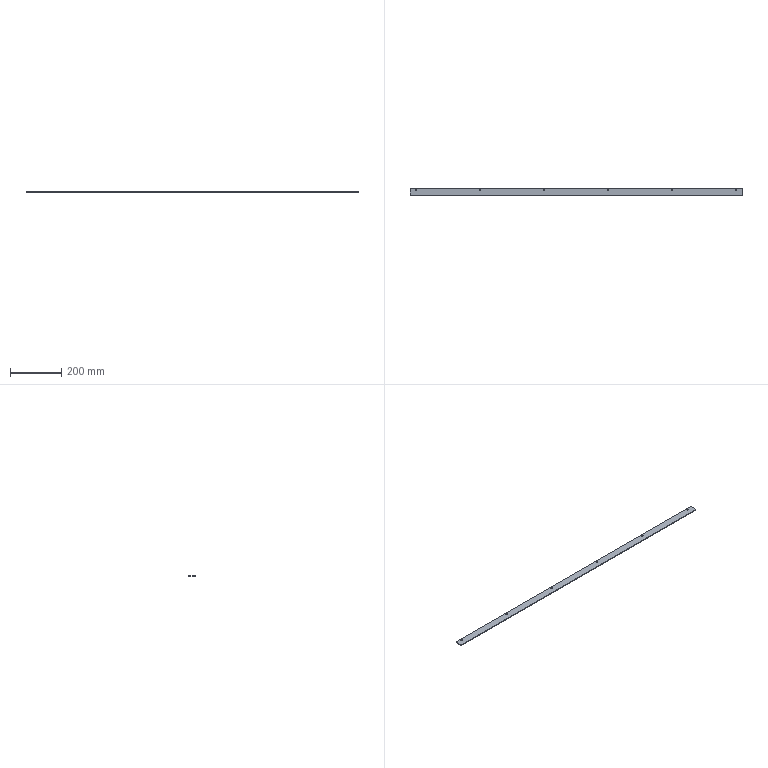Part | NX | features BREP 1 | 1 solid | 34 faces | box 1300 x 30 x 3 mm | volume 116367 mm3 | cone 12 | cylinder 12 | plane 10 | commonest cylinder face diameters 4.8 x12
STEP:
#1=CARTESIAN_POINT('',(648.,-15.,3.));
#2=VERTEX_POINT('',#1);
#3=CARTESIAN_POINT('',(650.,-13.,3.));
#4=VERTEX_POINT('',#3);
#5=CARTESIAN_POINT('',(331.5,-331.5,3.));
#6=DIRECTION('',(0.7071,0.7071,0.));
#7=VECTOR('',#6,1000.);
#8=LINE('',#5,#7);
#9=EDGE_CURVE('',#2,#4,#8,.T.);
#10=ORIENTED_EDGE('',*,*,#9,.F.);
#11=CARTESIAN_POINT('',(648.,-15.,0.));
#12=VERTEX_POINT('',#11);
#13=CARTESIAN_POINT('',(648.,-15.,3.));
#14=DIRECTION('',(0.,0.,1.));
#15=VECTOR('',#14,1000.);
#16=LINE('',#13,#15);
#17=EDGE_CURVE('',#12,#2,#16,.T.);
#18=ORIENTED_EDGE('',*,*,#17,.F.);
#19=CARTESIAN_POINT('',(650.,-13.,0.));
#20=VERTEX_POINT('',#19);
#21=CARTESIAN_POINT('',(650.,-13.,0.));
#22=DIRECTION('',(-0.7071,-0.7071,0.));
#23=VECTOR('',#22,1000.);
#24=LINE('',#21,#23);
#25=EDGE_CURVE('',#20,#12,#24,.T.);
#26=ORIENTED_EDGE('',*,*,#25,.F.);
#27=CARTESIAN_POINT('',(650.,-13.,3.));
#28=DIRECTION('',(0.,0.,-1.));
#29=VECTOR('',#28,1000.);
#30=LINE('',#27,#29);
#31=EDGE_CURVE('',#4,#20,#30,.T.);
#32=ORIENTED_EDGE('',*,*,#31,.F.);
#33=EDGE_LOOP('',(#10,#18,#26,#32));
#34=FACE_BOUND('',#33,.T.);
#35=CARTESIAN_POINT('',(650.,-13.,3.));
#36=DIRECTION('',(-0.7071,0.7071,0.));
#37=DIRECTION('',(0.,0.,-1.));
#38=AXIS2_PLACEMENT_3D('',#35,#36,#37);
#39=PLANE('',#38);
#40=ADVANCED_FACE('',(#34),#39,.F.);
#41=CARTESIAN_POINT('',(650.,13.,3.));
#42=VERTEX_POINT('',#41);
#43=CARTESIAN_POINT('',(648.,15.,3.));
#44=VERTEX_POINT('',#43);
#45=CARTESIAN_POINT('',(331.5,331.5,3.));
#46=DIRECTION('',(-0.7071,0.7071,0.));
#47=VECTOR('',#46,1000.);
#48=LINE('',#45,#47);
#49=EDGE_CURVE('',#42,#44,#48,.T.);
#50=ORIENTED_EDGE('',*,*,#49,.F.);
#51=CARTESIAN_POINT('',(650.,13.,0.));
#52=VERTEX_POINT('',#51);
#53=CARTESIAN_POINT('',(650.,13.,3.));
#54=DIRECTION('',(0.,0.,1.));
#55=VECTOR('',#54,1000.);
#56=LINE('',#53,#55);
#57=EDGE_CURVE('',#52,#42,#56,.T.);
#58=ORIENTED_EDGE('',*,*,#57,.F.);
#59=CARTESIAN_POINT('',(648.,15.,0.));
#60=VERTEX_POINT('',#59);
#61=CARTESIAN_POINT('',(648.,15.,0.));
#62=DIRECTION('',(0.7071,-0.7071,0.));
#63=VECTOR('',#62,1000.);
#64=LINE('',#61,#63);
#65=EDGE_CURVE('',#60,#52,#64,.T.);
#66=ORIENTED_EDGE('',*,*,#65,.F.);
#67=CARTESIAN_POINT('',(648.,15.,3.));
#68=DIRECTION('',(0.,0.,-1.));
#69=VECTOR('',#68,1000.);
#70=LINE('',#67,#69);
#71=EDGE_CURVE('',#44,#60,#70,.T.);
#72=ORIENTED_EDGE('',*,*,#71,.F.);
#73=EDGE_LOOP('',(#50,#58,#66,#72));
#74=FACE_BOUND('',#73,.T.);
#75=CARTESIAN_POINT('',(648.,15.,3.));
#76=DIRECTION('',(-0.7071,-0.7071,0.));
#77=DIRECTION('',(0.,0.,-1.));
#78=AXIS2_PLACEMENT_3D('',#75,#76,#77);
#79=PLANE('',#78);
#80=ADVANCED_FACE('',(#74),#79,.F.);
#81=CARTESIAN_POINT('',(-650.,-13.,3.));
#82=VERTEX_POINT('',#81);
#83=CARTESIAN_POINT('',(-648.,-15.,3.));
#84=VERTEX_POINT('',#83);
#85=CARTESIAN_POINT('',(-331.5,-331.5,3.));
#86=DIRECTION('',(0.7071,-0.7071,0.));
#87=VECTOR('',#86,1000.);
#88=LINE('',#85,#87);
#89=EDGE_CURVE('',#82,#84,#88,.T.);
#90=ORIENTED_EDGE('',*,*,#89,.F.);
#91=CARTESIAN_POINT('',(-650.,-13.,0.));
#92=VERTEX_POINT('',#91);
#93=CARTESIAN_POINT('',(-650.,-13.,3.));
#94=DIRECTION('',(0.,0.,1.));
#95=VECTOR('',#94,1000.);
#96=LINE('',#93,#95);
#97=EDGE_CURVE('',#92,#82,#96,.T.);
#98=ORIENTED_EDGE('',*,*,#97,.F.);
#99=CARTESIAN_POINT('',(-648.,-15.,0.));
#100=VERTEX_POINT('',#99);
#101=CARTESIAN_POINT('',(-648.,-15.,0.));
#102=DIRECTION('',(-0.7071,0.7071,0.));
#103=VECTOR('',#102,1000.);
#104=LINE('',#101,#103);
#105=EDGE_CURVE('',#100,#92,#104,.T.);
#106=ORIENTED_EDGE('',*,*,#105,.F.);
#107=CARTESIAN_POINT('',(-648.,-15.,3.));
#108=DIRECTION('',(0.,0.,-1.));
#109=VECTOR('',#108,1000.);
#110=LINE('',#107,#109);
#111=EDGE_CURVE('',#84,#100,#110,.T.);
#112=ORIENTED_EDGE('',*,*,#111,.F.);
#113=EDGE_LOOP('',(#90,#98,#106,#112));
#114=FACE_BOUND('',#113,.T.);
#115=CARTESIAN_POINT('',(-648.,-15.,3.));
#116=DIRECTION('',(0.7071,0.7071,0.));
#117=DIRECTION('',(0.,0.,-1.));
#118=AXIS2_PLACEMENT_3D('',#115,#116,#117);
#119=PLANE('',#118);
#120=ADVANCED_FACE('',(#114),#119,.F.);
#121=CARTESIAN_POINT('',(-648.,15.,3.));
#122=VERTEX_POINT('',#121);
#123=CARTESIAN_POINT('',(-650.,13.,3.));
#124=VERTEX_POINT('',#123);
#125=CARTESIAN_POINT('',(-331.5,331.5,3.));
#126=DIRECTION('',(-0.7071,-0.7071,0.));
#127=VECTOR('',#126,1000.);
#128=LINE('',#125,#127);
#129=EDGE_CURVE('',#122,#124,#128,.T.);
#130=ORIENTED_EDGE('',*,*,#129,.F.);
#131=CARTESIAN_POINT('',(-648.,15.,0.));
#132=VERTEX_POINT('',#131);
#133=CARTESIAN_POINT('',(-648.,15.,3.));
#134=DIRECTION('',(0.,0.,1.));
#135=VECTOR('',#134,1000.);
#136=LINE('',#133,#135);
#137=EDGE_CURVE('',#132,#122,#136,.T.);
#138=ORIENTED_EDGE('',*,*,#137,.F.);
#139=CARTESIAN_POINT('',(-650.,13.,0.));
#140=VERTEX_POINT('',#139);
#141=CARTESIAN_POINT('',(-650.,13.,0.));
#142=DIRECTION('',(0.7071,0.7071,0.));
#143=VECTOR('',#142,1000.);
#144=LINE('',#141,#143);
#145=EDGE_CURVE('',#140,#132,#144,.T.);
#146=ORIENTED_EDGE('',*,*,#145,.F.);
#147=CARTESIAN_POINT('',(-650.,13.,3.));
#148=DIRECTION('',(0.,0.,-1.));
#149=VECTOR('',#148,1000.);
#150=LINE('',#147,#149);
#151=EDGE_CURVE('',#124,#140,#150,.T.);
#152=ORIENTED_EDGE('',*,*,#151,.F.);
#153=EDGE_LOOP('',(#130,#138,#146,#152));
#154=FACE_BOUND('',#153,.T.);
#155=CARTESIAN_POINT('',(-650.,13.,3.));
#156=DIRECTION('',(0.7071,-0.7071,0.));
#157=DIRECTION('',(0.,0.,-1.));
#158=AXIS2_PLACEMENT_3D('',#155,#156,#157);
#159=PLANE('',#158);
#160=ADVANCED_FACE('',(#154),#159,.F.);
#161=CARTESIAN_POINT('',(627.4,9.,2.19));
#162=VERTEX_POINT('',#161);
#163=CARTESIAN_POINT('',(629.59,9.,0.));
#164=VERTEX_POINT('',#163);
#165=CARTESIAN_POINT('',(629.59,9.,0.));
#166=DIRECTION('',(0.7071,0.,-0.7071));
#167=VECTOR('',#166,1000.);
#168=LINE('',#165,#167);
#169=EDGE_CURVE('',#162,#164,#168,.T.);
#170=ORIENTED_EDGE('',*,*,#169,.F.);
#171=CARTESIAN_POINT('',(622.6,9.,2.19));
#172=VERTEX_POINT('',#171);
#173=CARTESIAN_POINT('',(625.,9.,2.19));
#174=DIRECTION('',(0.,0.,-1.));
#175=DIRECTION('',(-1.,0.,0.));
#176=AXIS2_PLACEMENT_3D('',#173,#174,#175);
#177=CIRCLE('',#176,2.4);
#178=EDGE_CURVE('',#172,#162,#177,.T.);
#179=ORIENTED_EDGE('',*,*,#178,.F.);
#180=CARTESIAN_POINT('',(620.41,9.,0.));
#181=VERTEX_POINT('',#180);
#182=CARTESIAN_POINT('',(620.41,9.,0.));
#183=DIRECTION('',(-0.7071,0.,-0.7071));
#184=VECTOR('',#183,1000.);
#185=LINE('',#182,#184);
#186=EDGE_CURVE('',#172,#181,#185,.T.);
#187=ORIENTED_EDGE('',*,*,#186,.T.);
#188=CARTESIAN_POINT('',(625.,9.,0.));
#189=DIRECTION('',(0.,0.,-1.));
#190=DIRECTION('',(-1.,0.,0.));
#191=AXIS2_PLACEMENT_3D('',#188,#189,#190);
#192=CIRCLE('',#191,4.59);
#193=EDGE_CURVE('',#181,#164,#192,.T.);
#194=ORIENTED_EDGE('',*,*,#193,.T.);
#195=EDGE_LOOP('',(#170,#179,#187,#194));
#196=FACE_BOUND('',#195,.T.);
#197=CARTESIAN_POINT('',(625.,9.,0.));
#198=DIRECTION('',(0.,0.,-1.));
#199=DIRECTION('',(-1.,0.,0.));
#200=AXIS2_PLACEMENT_3D('',#197,#198,#199);
#201=CONICAL_SURFACE('',#200,4.59,0.7854);
#202=ADVANCED_FACE('',(#196),#201,.F.);
#203=CARTESIAN_POINT('',(627.4,9.,3.));
#204=VERTEX_POINT('',#203);
#205=CARTESIAN_POINT('',(627.4,9.,0.));
#206=DIRECTION('',(0.,0.,-1.));
#207=VECTOR('',#206,1000.);
#208=LINE('',#205,#207);
#209=EDGE_CURVE('',#204,#162,#208,.T.);
#210=ORIENTED_EDGE('',*,*,#209,.F.);
#211=CARTESIAN_POINT('',(622.6,9.,3.));
#212=VERTEX_POINT('',#211);
#213=CARTESIAN_POINT('',(625.,9.,3.));
#214=DIRECTION('',(0.,0.,-1.));
#215=DIRECTION('',(-1.,0.,0.));
#216=AXIS2_PLACEMENT_3D('',#213,#214,#215);
#217=CIRCLE('',#216,2.4);
#218=EDGE_CURVE('',#212,#204,#217,.T.);
#219=ORIENTED_EDGE('',*,*,#218,.F.);
#220=CARTESIAN_POINT('',(622.6,9.,0.));
#221=DIRECTION('',(0.,0.,-1.));
#222=VECTOR('',#221,1000.);
#223=LINE('',#220,#222);
#224=EDGE_CURVE('',#212,#172,#223,.T.);
#225=ORIENTED_EDGE('',*,*,#224,.T.);
#226=ORIENTED_EDGE('',*,*,#178,.T.);
#227=EDGE_LOOP('',(#210,#219,#225,#226));
#228=FACE_BOUND('',#227,.T.);
#229=CARTESIAN_POINT('',(625.,9.,0.));
#230=DIRECTION('',(0.,0.,-1.));
#231=DIRECTION('',(-1.,0.,0.));
#232=AXIS2_PLACEMENT_3D('',#229,#230,#231);
#233=CYLINDRICAL_SURFACE('',#232,2.4);
#234=ADVANCED_FACE('',(#228),#233,.F.);
#235=CARTESIAN_POINT('',(377.4,9.,2.19));
#236=VERTEX_POINT('',#235);
#237=CARTESIAN_POINT('',(379.59,9.,0.));
#238=VERTEX_POINT('',#237);
#239=CARTESIAN_POINT('',(379.59,9.,0.));
#240=DIRECTION('',(0.7071,0.,-0.7071));
#241=VECTOR('',#240,1000.);
#242=LINE('',#239,#241);
#243=EDGE_CURVE('',#236,#238,#242,.T.);
#244=ORIENTED_EDGE('',*,*,#243,.F.);
#245=CARTESIAN_POINT('',(372.6,9.,2.19));
#246=VERTEX_POINT('',#245);
#247=CARTESIAN_POINT('',(375.,9.,2.19));
#248=DIRECTION('',(0.,0.,-1.));
#249=DIRECTION('',(-1.,0.,0.));
#250=AXIS2_PLACEMENT_3D('',#247,#248,#249);
#251=CIRCLE('',#250,2.4);
#252=EDGE_CURVE('',#246,#236,#251,.T.);
#253=ORIENTED_EDGE('',*,*,#252,.F.);
#254=CARTESIAN_POINT('',(370.41,9.,0.));
#255=VERTEX_POINT('',#254);
#256=CARTESIAN_POINT('',(370.41,9.,0.));
#257=DIRECTION('',(-0.7071,0.,-0.7071));
#258=VECTOR('',#257,1000.);
#259=LINE('',#256,#258);
#260=EDGE_CURVE('',#246,#255,#259,.T.);
#261=ORIENTED_EDGE('',*,*,#260,.T.);
#262=CARTESIAN_POINT('',(375.,9.,0.));
#263=DIRECTION('',(0.,0.,-1.));
#264=DIRECTION('',(-1.,0.,0.));
#265=AXIS2_PLACEMENT_3D('',#262,#263,#264);
#266=CIRCLE('',#265,4.59);
#267=EDGE_CURVE('',#255,#238,#266,.T.);
#268=ORIENTED_EDGE('',*,*,#267,.T.);
#269=EDGE_LOOP('',(#244,#253,#261,#268));
#270=FACE_BOUND('',#269,.T.);
#271=CARTESIAN_POINT('',(375.,9.,0.));
#272=DIRECTION('',(0.,0.,-1.));
#273=DIRECTION('',(-1.,0.,0.));
#274=AXIS2_PLACEMENT_3D('',#271,#272,#273);
#275=CONICAL_SURFACE('',#274,4.59,0.7854);
#276=ADVANCED_FACE('',(#270),#275,.F.);
#277=CARTESIAN_POINT('',(377.4,9.,3.));
#278=VERTEX_POINT('',#277);
#279=CARTESIAN_POINT('',(377.4,9.,0.));
#280=DIRECTION('',(0.,0.,-1.));
#281=VECTOR('',#280,1000.);
#282=LINE('',#279,#281);
#283=EDGE_CURVE('',#278,#236,#282,.T.);
#284=ORIENTED_EDGE('',*,*,#283,.F.);
#285=CARTESIAN_POINT('',(372.6,9.,3.));
#286=VERTEX_POINT('',#285);
#287=CARTESIAN_POINT('',(375.,9.,3.));
#288=DIRECTION('',(0.,0.,-1.));
#289=DIRECTION('',(-1.,0.,0.));
#290=AXIS2_PLACEMENT_3D('',#287,#288,#289);
#291=CIRCLE('',#290,2.4);
#292=EDGE_CURVE('',#286,#278,#291,.T.);
#293=ORIENTED_EDGE('',*,*,#292,.F.);
#294=CARTESIAN_POINT('',(372.6,9.,0.));
#295=DIRECTION('',(0.,0.,-1.));
#296=VECTOR('',#295,1000.);
#297=LINE('',#294,#296);
#298=EDGE_CURVE('',#286,#246,#297,.T.);
#299=ORIENTED_EDGE('',*,*,#298,.T.);
#300=ORIENTED_EDGE('',*,*,#252,.T.);
#301=EDGE_LOOP('',(#284,#293,#299,#300));
#302=FACE_BOUND('',#301,.T.);
#303=CARTESIAN_POINT('',(375.,9.,0.));
#304=DIRECTION('',(0.,0.,-1.));
#305=DIRECTION('',(-1.,0.,0.));
#306=AXIS2_PLACEMENT_3D('',#303,#304,#305);
#307=CYLINDRICAL_SURFACE('',#306,2.4);
#308=ADVANCED_FACE('',(#302),#307,.F.);
#309=CARTESIAN_POINT('',(127.4,9.,2.19));
#310=VERTEX_POINT('',#309);
#311=CARTESIAN_POINT('',(129.59,9.,0.));
#312=VERTEX_POINT('',#311);
#313=CARTESIAN_POINT('',(129.59,9.,0.));
#314=DIRECTION('',(0.7071,0.,-0.7071));
#315=VECTOR('',#314,1000.);
#316=LINE('',#313,#315);
#317=EDGE_CURVE('',#310,#312,#316,.T.);
#318=ORIENTED_EDGE('',*,*,#317,.F.);
#319=CARTESIAN_POINT('',(122.6,9.,2.19));
#320=VERTEX_POINT('',#319);
#321=CARTESIAN_POINT('',(125.,9.,2.19));
#322=DIRECTION('',(0.,0.,-1.));
#323=DIRECTION('',(-1.,0.,0.));
#324=AXIS2_PLACEMENT_3D('',#321,#322,#323);
#325=CIRCLE('',#324,2.4);
#326=EDGE_CURVE('',#320,#310,#325,.T.);
#327=ORIENTED_EDGE('',*,*,#326,.F.);
#328=CARTESIAN_POINT('',(120.41,9.,0.));
#329=VERTEX_POINT('',#328);
#330=CARTESIAN_POINT('',(120.41,9.,0.));
#331=DIRECTION('',(-0.7071,0.,-0.7071));
#332=VECTOR('',#331,1000.);
#333=LINE('',#330,#332);
#334=EDGE_CURVE('',#320,#329,#333,.T.);
#335=ORIENTED_EDGE('',*,*,#334,.T.);
#336=CARTESIAN_POINT('',(125.,9.,0.));
#337=DIRECTION('',(0.,0.,-1.));
#338=DIRECTION('',(-1.,0.,0.));
#339=AXIS2_PLACEMENT_3D('',#336,#337,#338);
#340=CIRCLE('',#339,4.59);
#341=EDGE_CURVE('',#329,#312,#340,.T.);
#342=ORIENTED_EDGE('',*,*,#341,.T.);
#343=EDGE_LOOP('',(#318,#327,#335,#342));
#344=FACE_BOUND('',#343,.T.);
#345=CARTESIAN_POINT('',(125.,9.,0.));
#346=DIRECTION('',(0.,0.,-1.));
#347=DIRECTION('',(-1.,0.,0.));
#348=AXIS2_PLACEMENT_3D('',#345,#346,#347);
#349=CONICAL_SURFACE('',#348,4.59,0.7854);
#350=ADVANCED_FACE('',(#344),#349,.F.);
#351=CARTESIAN_POINT('',(127.4,9.,3.));
#352=VERTEX_POINT('',#351);
#353=CARTESIAN_POINT('',(127.4,9.,0.));
#354=DIRECTION('',(0.,0.,-1.));
#355=VECTOR('',#354,1000.);
#356=LINE('',#353,#355);
#357=EDGE_CURVE('',#352,#310,#356,.T.);
#358=ORIENTED_EDGE('',*,*,#357,.F.);
#359=CARTESIAN_POINT('',(122.6,9.,3.));
#360=VERTEX_POINT('',#359);
#361=CARTESIAN_POINT('',(125.,9.,3.));
#362=DIRECTION('',(0.,0.,-1.));
#363=DIRECTION('',(-1.,0.,0.));
#364=AXIS2_PLACEMENT_3D('',#361,#362,#363);
#365=CIRCLE('',#364,2.4);
#366=EDGE_CURVE('',#360,#352,#365,.T.);
#367=ORIENTED_EDGE('',*,*,#366,.F.);
#368=CARTESIAN_POINT('',(122.6,9.,0.));
#369=DIRECTION('',(0.,0.,-1.));
#370=VECTOR('',#369,1000.);
#371=LINE('',#368,#370);
#372=EDGE_CURVE('',#360,#320,#371,.T.);
#373=ORIENTED_EDGE('',*,*,#372,.T.);
#374=ORIENTED_EDGE('',*,*,#326,.T.);
#375=EDGE_LOOP('',(#358,#367,#373,#374));
#376=FACE_BOUND('',#375,.T.);
#377=CARTESIAN_POINT('',(125.,9.,0.));
#378=DIRECTION('',(0.,0.,-1.));
#379=DIRECTION('',(-1.,0.,0.));
#380=AXIS2_PLACEMENT_3D('',#377,#378,#379);
#381=CYLINDRICAL_SURFACE('',#380,2.4);
#382=ADVANCED_FACE('',(#376),#381,.F.);
#383=CARTESIAN_POINT('',(-122.6,9.,2.19));
#384=VERTEX_POINT('',#383);
#385=CARTESIAN_POINT('',(-120.41,9.,0.));
#386=VERTEX_POINT('',#385);
#387=CARTESIAN_POINT('',(-120.41,9.,0.));
#388=DIRECTION('',(0.7071,0.,-0.7071));
#389=VECTOR('',#388,1000.);
#390=LINE('',#387,#389);
#391=EDGE_CURVE('',#384,#386,#390,.T.);
#392=ORIENTED_EDGE('',*,*,#391,.F.);
#393=CARTESIAN_POINT('',(-127.4,9.,2.19));
#394=VERTEX_POINT('',#393);
#395=CARTESIAN_POINT('',(-125.,9.,2.19));
#396=DIRECTION('',(0.,0.,-1.));
#397=DIRECTION('',(-1.,0.,0.));
#398=AXIS2_PLACEMENT_3D('',#395,#396,#397);
#399=CIRCLE('',#398,2.4);
#400=EDGE_CURVE('',#394,#384,#399,.T.);
#401=ORIENTED_EDGE('',*,*,#400,.F.);
#402=CARTESIAN_POINT('',(-129.59,9.,0.));
#403=VERTEX_POINT('',#402);
#404=CARTESIAN_POINT('',(-129.59,9.,0.));
#405=DIRECTION('',(-0.7071,0.,-0.7071));
#406=VECTOR('',#405,1000.);
#407=LINE('',#404,#406);
#408=EDGE_CURVE('',#394,#403,#407,.T.);
#409=ORIENTED_EDGE('',*,*,#408,.T.);
#410=CARTESIAN_POINT('',(-125.,9.,0.));
#411=DIRECTION('',(0.,0.,-1.));
#412=DIRECTION('',(-1.,0.,0.));
#413=AXIS2_PLACEMENT_3D('',#410,#411,#412);
#414=CIRCLE('',#413,4.59);
#415=EDGE_CURVE('',#403,#386,#414,.T.);
#416=ORIENTED_EDGE('',*,*,#415,.T.);
#417=EDGE_LOOP('',(#392,#401,#409,#416));
#418=FACE_BOUND('',#417,.T.);
#419=CARTESIAN_POINT('',(-125.,9.,0.));
#420=DIRECTION('',(0.,0.,-1.));
#421=DIRECTION('',(-1.,0.,0.));
#422=AXIS2_PLACEMENT_3D('',#419,#420,#421);
#423=CONICAL_SURFACE('',#422,4.59,0.7854);
#424=ADVANCED_FACE('',(#418),#423,.F.);
#425=CARTESIAN_POINT('',(-122.6,9.,3.));
#426=VERTEX_POINT('',#425);
#427=CARTESIAN_POINT('',(-122.6,9.,0.));
#428=DIRECTION('',(0.,0.,-1.));
#429=VECTOR('',#428,1000.);
#430=LINE('',#427,#429);
#431=EDGE_CURVE('',#426,#384,#430,.T.);
#432=ORIENTED_EDGE('',*,*,#431,.F.);
#433=CARTESIAN_POINT('',(-127.4,9.,3.));
#434=VERTEX_POINT('',#433);
#435=CARTESIAN_POINT('',(-125.,9.,3.));
#436=DIRECTION('',(0.,0.,-1.));
#437=DIRECTION('',(-1.,0.,0.));
#438=AXIS2_PLACEMENT_3D('',#435,#436,#437);
#439=CIRCLE('',#438,2.4);
#440=EDGE_CURVE('',#434,#426,#439,.T.);
#441=ORIENTED_EDGE('',*,*,#440,.F.);
#442=CARTESIAN_POINT('',(-127.4,9.,0.));
#443=DIRECTION('',(0.,0.,-1.));
#444=VECTOR('',#443,1000.);
#445=LINE('',#442,#444);
#446=EDGE_CURVE('',#434,#394,#445,.T.);
#447=ORIENTED_EDGE('',*,*,#446,.T.);
#448=ORIENTED_EDGE('',*,*,#400,.T.);
#449=EDGE_LOOP('',(#432,#441,#447,#448));
#450=FACE_BOUND('',#449,.T.);
#451=CARTESIAN_POINT('',(-125.,9.,0.));
#452=DIRECTION('',(0.,0.,-1.));
#453=DIRECTION('',(-1.,0.,0.));
#454=AXIS2_PLACEMENT_3D('',#451,#452,#453);
#455=CYLINDRICAL_SURFACE('',#454,2.4);
#456=ADVANCED_FACE('',(#450),#455,.F.);
#457=CARTESIAN_POINT('',(-372.6,9.,2.19));
#458=VERTEX_POINT('',#457);
#459=CARTESIAN_POINT('',(-370.41,9.,0.));
#460=VERTEX_POINT('',#459);
#461=CARTESIAN_POINT('',(-370.41,9.,0.));
#462=DIRECTION('',(0.7071,0.,-0.7071));
#463=VECTOR('',#462,1000.);
#464=LINE('',#461,#463);
#465=EDGE_CURVE('',#458,#460,#464,.T.);
#466=ORIENTED_EDGE('',*,*,#465,.F.);
#467=CARTESIAN_POINT('',(-377.4,9.,2.19));
#468=VERTEX_POINT('',#467);
#469=CARTESIAN_POINT('',(-375.,9.,2.19));
#470=DIRECTION('',(0.,0.,-1.));
#471=DIRECTION('',(-1.,0.,0.));
#472=AXIS2_PLACEMENT_3D('',#469,#470,#471);
#473=CIRCLE('',#472,2.4);
#474=EDGE_CURVE('',#468,#458,#473,.T.);
#475=ORIENTED_EDGE('',*,*,#474,.F.);
#476=CARTESIAN_POINT('',(-379.59,9.,0.));
#477=VERTEX_POINT('',#476);
#478=CARTESIAN_POINT('',(-379.59,9.,0.));
#479=DIRECTION('',(-0.7071,0.,-0.7071));
#480=VECTOR('',#479,1000.);
#481=LINE('',#478,#480);
#482=EDGE_CURVE('',#468,#477,#481,.T.);
#483=ORIENTED_EDGE('',*,*,#482,.T.);
#484=CARTESIAN_POINT('',(-375.,9.,0.));
#485=DIRECTION('',(0.,0.,-1.));
#486=DIRECTION('',(-1.,0.,0.));
#487=AXIS2_PLACEMENT_3D('',#484,#485,#486);
#488=CIRCLE('',#487,4.59);
#489=EDGE_CURVE('',#477,#460,#488,.T.);
#490=ORIENTED_EDGE('',*,*,#489,.T.);
#491=EDGE_LOOP('',(#466,#475,#483,#490));
#492=FACE_BOUND('',#491,.T.);
#493=CARTESIAN_POINT('',(-375.,9.,0.));
#494=DIRECTION('',(0.,0.,-1.));
#495=DIRECTION('',(-1.,0.,0.));
#496=AXIS2_PLACEMENT_3D('',#493,#494,#495);
#497=CONICAL_SURFACE('',#496,4.59,0.7854);
#498=ADVANCED_FACE('',(#492),#497,.F.);
#499=CARTESIAN_POINT('',(-372.6,9.,3.));
#500=VERTEX_POINT('',#499);
#501=CARTESIAN_POINT('',(-372.6,9.,0.));
#502=DIRECTION('',(0.,0.,-1.));
#503=VECTOR('',#502,1000.);
#504=LINE('',#501,#503);
#505=EDGE_CURVE('',#500,#458,#504,.T.);
#506=ORIENTED_EDGE('',*,*,#505,.F.);
#507=CARTESIAN_POINT('',(-377.4,9.,3.));
#508=VERTEX_POINT('',#507);
#509=CARTESIAN_POINT('',(-375.,9.,3.));
#510=DIRECTION('',(0.,0.,-1.));
#511=DIRECTION('',(-1.,0.,0.));
#512=AXIS2_PLACEMENT_3D('',#509,#510,#511);
#513=CIRCLE('',#512,2.4);
#514=EDGE_CURVE('',#508,#500,#513,.T.);
#515=ORIENTED_EDGE('',*,*,#514,.F.);
#516=CARTESIAN_POINT('',(-377.4,9.,0.));
#517=DIRECTION('',(0.,0.,-1.));
#518=VECTOR('',#517,1000.);
#519=LINE('',#516,#518);
#520=EDGE_CURVE('',#508,#468,#519,.T.);
#521=ORIENTED_EDGE('',*,*,#520,.T.);
#522=ORIENTED_EDGE('',*,*,#474,.T.);
#523=EDGE_LOOP('',(#506,#515,#521,#522));
#524=FACE_BOUND('',#523,.T.);
#525=CARTESIAN_POINT('',(-375.,9.,0.));
#526=DIRECTION('',(0.,0.,-1.));
#527=DIRECTION('',(-1.,0.,0.));
#528=AXIS2_PLACEMENT_3D('',#525,#526,#527);
#529=CYLINDRICAL_SURFACE('',#528,2.4);
#530=ADVANCED_FACE('',(#524),#529,.F.);
#531=CARTESIAN_POINT('',(-622.6,9.,2.19));
#532=VERTEX_POINT('',#531);
#533=CARTESIAN_POINT('',(-620.41,9.,0.));
#534=VERTEX_POINT('',#533);
#535=CARTESIAN_POINT('',(-620.41,9.,0.));
#536=DIRECTION('',(0.7071,0.,-0.7071));
#537=VECTOR('',#536,1000.);
#538=LINE('',#535,#537);
#539=EDGE_CURVE('',#532,#534,#538,.T.);
#540=ORIENTED_EDGE('',*,*,#539,.F.);
#541=CARTESIAN_POINT('',(-627.4,9.,2.19));
#542=VERTEX_POINT('',#541);
#543=CARTESIAN_POINT('',(-625.,9.,2.19));
#544=DIRECTION('',(0.,0.,-1.));
#545=DIRECTION('',(-1.,0.,0.));
#546=AXIS2_PLACEMENT_3D('',#543,#544,#545);
#547=CIRCLE('',#546,2.4);
#548=EDGE_CURVE('',#542,#532,#547,.T.);
#549=ORIENTED_EDGE('',*,*,#548,.F.);
#550=CARTESIAN_POINT('',(-629.59,9.,0.));
#551=VERTEX_POINT('',#550);
#552=CARTESIAN_POINT('',(-629.59,9.,0.));
#553=DIRECTION('',(-0.7071,0.,-0.7071));
#554=VECTOR('',#553,1000.);
#555=LINE('',#552,#554);
#556=EDGE_CURVE('',#542,#551,#555,.T.);
#557=ORIENTED_EDGE('',*,*,#556,.T.);
#558=CARTESIAN_POINT('',(-625.,9.,0.));
#559=DIRECTION('',(0.,0.,-1.));
#560=DIRECTION('',(-1.,0.,0.));
#561=AXIS2_PLACEMENT_3D('',#558,#559,#560);
#562=CIRCLE('',#561,4.59);
#563=EDGE_CURVE('',#551,#534,#562,.T.);
#564=ORIENTED_EDGE('',*,*,#563,.T.);
#565=EDGE_LOOP('',(#540,#549,#557,#564));
#566=FACE_BOUND('',#565,.T.);
#567=CARTESIAN_POINT('',(-625.,9.,0.));
#568=DIRECTION('',(0.,0.,-1.));
#569=DIRECTION('',(-1.,0.,0.));
#570=AXIS2_PLACEMENT_3D('',#567,#568,#569);
#571=CONICAL_SURFACE('',#570,4.59,0.7854);
#572=ADVANCED_FACE('',(#566),#571,.F.);
#573=CARTESIAN_POINT('',(-622.6,9.,3.));
#574=VERTEX_POINT('',#573);
#575=CARTESIAN_POINT('',(-622.6,9.,0.));
#576=DIRECTION('',(0.,0.,-1.));
#577=VECTOR('',#576,1000.);
#578=LINE('',#575,#577);
#579=EDGE_CURVE('',#574,#532,#578,.T.);
#580=ORIENTED_EDGE('',*,*,#579,.F.);
#581=CARTESIAN_POINT('',(-627.4,9.,3.));
#582=VERTEX_POINT('',#581);
#583=CARTESIAN_POINT('',(-625.,9.,3.));
#584=DIRECTION('',(0.,0.,-1.));
#585=DIRECTION('',(-1.,0.,0.));
#586=AXIS2_PLACEMENT_3D('',#583,#584,#585);
#587=CIRCLE('',#586,2.4);
#588=EDGE_CURVE('',#582,#574,#587,.T.);
#589=ORIENTED_EDGE('',*,*,#588,.F.);
#590=CARTESIAN_POINT('',(-627.4,9.,0.));
#591=DIRECTION('',(0.,0.,-1.));
#592=VECTOR('',#591,1000.);
#593=LINE('',#590,#592);
#594=EDGE_CURVE('',#582,#542,#593,.T.);
#595=ORIENTED_EDGE('',*,*,#594,.T.);
#596=ORIENTED_EDGE('',*,*,#548,.T.);
#597=EDGE_LOOP('',(#580,#589,#595,#596));
#598=FACE_BOUND('',#597,.T.);
#599=CARTESIAN_POINT('',(-625.,9.,0.));
#600=DIRECTION('',(0.,0.,-1.));
#601=DIRECTION('',(-1.,0.,0.));
#602=AXIS2_PLACEMENT_3D('',#599,#600,#601);
#603=CYLINDRICAL_SURFACE('',#602,2.4);
#604=ADVANCED_FACE('',(#598),#603,.F.);
#605=CARTESIAN_POINT('',(-650.,-15.,0.));
#606=DIRECTION('',(0.,-1.,0.));
#607=VECTOR('',#606,1000.);
#608=LINE('',#605,#607);
#609=EDGE_CURVE('',#140,#92,#608,.T.);
#610=ORIENTED_EDGE('',*,*,#609,.F.);
#611=ORIENTED_EDGE('',*,*,#145,.T.);
#612=CARTESIAN_POINT('',(650.,15.,0.));
#613=DIRECTION('',(-1.,0.,0.));
#614=VECTOR('',#613,1000.);
#615=LINE('',#612,#614);
#616=EDGE_CURVE('',#60,#132,#615,.T.);
#617=ORIENTED_EDGE('',*,*,#616,.F.);
#618=ORIENTED_EDGE('',*,*,#65,.T.);
#619=CARTESIAN_POINT('',(650.,-15.,0.));
#620=DIRECTION('',(0.,1.,0.));
#621=VECTOR('',#620,1000.);
#622=LINE('',#619,#621);
#623=EDGE_CURVE('',#20,#52,#622,.T.);
#624=ORIENTED_EDGE('',*,*,#623,.F.);
#625=ORIENTED_EDGE('',*,*,#25,.T.);
#626=CARTESIAN_POINT('',(650.,-15.,0.));
#627=DIRECTION('',(1.,0.,0.));
#628=VECTOR('',#627,1000.);
#629=LINE('',#626,#628);
#630=EDGE_CURVE('',#100,#12,#629,.T.);
#631=ORIENTED_EDGE('',*,*,#630,.F.);
#632=ORIENTED_EDGE('',*,*,#105,.T.);
#633=EDGE_LOOP('',(#610,#611,#617,#618,#624,#625,#631,#632));
#634=FACE_BOUND('',#633,.T.);
#635=ORIENTED_EDGE('',*,*,#563,.F.);
#636=CARTESIAN_POINT('',(-625.,9.,0.));
#637=DIRECTION('',(0.,0.,-1.));
#638=DIRECTION('',(-1.,0.,0.));
#639=AXIS2_PLACEMENT_3D('',#636,#637,#638);
#640=CIRCLE('',#639,4.59);
#641=EDGE_CURVE('',#534,#551,#640,.T.);
#642=ORIENTED_EDGE('',*,*,#641,.F.);
#643=EDGE_LOOP('',(#635,#642));
#644=FACE_BOUND('',#643,.T.);
#645=ORIENTED_EDGE('',*,*,#489,.F.);
#646=CARTESIAN_POINT('',(-375.,9.,0.));
#647=DIRECTION('',(0.,0.,-1.));
#648=DIRECTION('',(-1.,0.,0.));
#649=AXIS2_PLACEMENT_3D('',#646,#647,#648);
#650=CIRCLE('',#649,4.59);
#651=EDGE_CURVE('',#460,#477,#650,.T.);
#652=ORIENTED_EDGE('',*,*,#651,.F.);
#653=EDGE_LOOP('',(#645,#652));
#654=FACE_BOUND('',#653,.T.);
#655=ORIENTED_EDGE('',*,*,#415,.F.);
#656=CARTESIAN_POINT('',(-125.,9.,0.));
#657=DIRECTION('',(0.,0.,-1.));
#658=DIRECTION('',(-1.,0.,0.));
#659=AXIS2_PLACEMENT_3D('',#656,#657,#658);
#660=CIRCLE('',#659,4.59);
#661=EDGE_CURVE('',#386,#403,#660,.T.);
#662=ORIENTED_EDGE('',*,*,#661,.F.);
#663=EDGE_LOOP('',(#655,#662));
#664=FACE_BOUND('',#663,.T.);
#665=ORIENTED_EDGE('',*,*,#341,.F.);
#666=CARTESIAN_POINT('',(125.,9.,0.));
#667=DIRECTION('',(0.,0.,-1.));
#668=DIRECTION('',(-1.,0.,0.));
#669=AXIS2_PLACEMENT_3D('',#666,#667,#668);
#670=CIRCLE('',#669,4.59);
#671=EDGE_CURVE('',#312,#329,#670,.T.);
#672=ORIENTED_EDGE('',*,*,#671,.F.);
#673=EDGE_LOOP('',(#665,#672));
#674=FACE_BOUND('',#673,.T.);
#675=ORIENTED_EDGE('',*,*,#267,.F.);
#676=CARTESIAN_POINT('',(375.,9.,0.));
#677=DIRECTION('',(0.,0.,-1.));
#678=DIRECTION('',(-1.,0.,0.));
#679=AXIS2_PLACEMENT_3D('',#676,#677,#678);
#680=CIRCLE('',#679,4.59);
#681=EDGE_CURVE('',#238,#255,#680,.T.);
#682=ORIENTED_EDGE('',*,*,#681,.F.);
#683=EDGE_LOOP('',(#675,#682));
#684=FACE_BOUND('',#683,.T.);
#685=ORIENTED_EDGE('',*,*,#193,.F.);
#686=CARTESIAN_POINT('',(625.,9.,0.));
#687=DIRECTION('',(0.,0.,-1.));
#688=DIRECTION('',(-1.,0.,0.));
#689=AXIS2_PLACEMENT_3D('',#686,#687,#688);
#690=CIRCLE('',#689,4.59);
#691=EDGE_CURVE('',#164,#181,#690,.T.);
#692=ORIENTED_EDGE('',*,*,#691,.F.);
#693=EDGE_LOOP('',(#685,#692));
#694=FACE_BOUND('',#693,.T.);
#695=CARTESIAN_POINT('',(0.,0.,0.));
#696=DIRECTION('',(0.,0.,1.));
#697=DIRECTION('',(1.,0.,0.));
#698=AXIS2_PLACEMENT_3D('',#695,#696,#697);
#699=PLANE('',#698);
#700=ADVANCED_FACE('',(#634,#644,#654,#664,#674,#684,#694),#699,.F.);
#701=CARTESIAN_POINT('',(650.,15.,3.));
#702=DIRECTION('',(-1.,0.,0.));
#703=VECTOR('',#702,1000.);
#704=LINE('',#701,#703);
#705=EDGE_CURVE('',#44,#122,#704,.T.);
#706=ORIENTED_EDGE('',*,*,#705,.T.);
#707=ORIENTED_EDGE('',*,*,#129,.T.);
#708=CARTESIAN_POINT('',(-650.,-15.,3.));
#709=DIRECTION('',(0.,-1.,0.));
#710=VECTOR('',#709,1000.);
#711=LINE('',#708,#710);
#712=EDGE_CURVE('',#124,#82,#711,.T.);
#713=ORIENTED_EDGE('',*,*,#712,.T.);
#714=ORIENTED_EDGE('',*,*,#89,.T.);
#715=CARTESIAN_POINT('',(650.,-15.,3.));
#716=DIRECTION('',(1.,0.,0.));
#717=VECTOR('',#716,1000.);
#718=LINE('',#715,#717);
#719=EDGE_CURVE('',#84,#2,#718,.T.);
#720=ORIENTED_EDGE('',*,*,#719,.T.);
#721=ORIENTED_EDGE('',*,*,#9,.T.);
#722=CARTESIAN_POINT('',(650.,-15.,3.));
#723=DIRECTION('',(0.,1.,0.));
#724=VECTOR('',#723,1000.);
#725=LINE('',#722,#724);
#726=EDGE_CURVE('',#4,#42,#725,.T.);
#727=ORIENTED_EDGE('',*,*,#726,.T.);
#728=ORIENTED_EDGE('',*,*,#49,.T.);
#729=EDGE_LOOP('',(#706,#707,#713,#714,#720,#721,#727,#728));
#730=FACE_BOUND('',#729,.T.);
#731=ORIENTED_EDGE('',*,*,#588,.T.);
#732=CARTESIAN_POINT('',(-625.,9.,3.));
#733=DIRECTION('',(0.,0.,-1.));
#734=DIRECTION('',(-1.,0.,0.));
#735=AXIS2_PLACEMENT_3D('',#732,#733,#734);
#736=CIRCLE('',#735,2.4);
#737=EDGE_CURVE('',#574,#582,#736,.T.);
#738=ORIENTED_EDGE('',*,*,#737,.T.);
#739=EDGE_LOOP('',(#731,#738));
#740=FACE_BOUND('',#739,.T.);
#741=ORIENTED_EDGE('',*,*,#514,.T.);
#742=CARTESIAN_POINT('',(-375.,9.,3.));
#743=DIRECTION('',(0.,0.,-1.));
#744=DIRECTION('',(-1.,0.,0.));
#745=AXIS2_PLACEMENT_3D('',#742,#743,#744);
#746=CIRCLE('',#745,2.4);
#747=EDGE_CURVE('',#500,#508,#746,.T.);
#748=ORIENTED_EDGE('',*,*,#747,.T.);
#749=EDGE_LOOP('',(#741,#748));
#750=FACE_BOUND('',#749,.T.);
#751=ORIENTED_EDGE('',*,*,#440,.T.);
#752=CARTESIAN_POINT('',(-125.,9.,3.));
#753=DIRECTION('',(0.,0.,-1.));
#754=DIRECTION('',(-1.,0.,0.));
#755=AXIS2_PLACEMENT_3D('',#752,#753,#754);
#756=CIRCLE('',#755,2.4);
#757=EDGE_CURVE('',#426,#434,#756,.T.);
#758=ORIENTED_EDGE('',*,*,#757,.T.);
#759=EDGE_LOOP('',(#751,#758));
#760=FACE_BOUND('',#759,.T.);
#761=ORIENTED_EDGE('',*,*,#366,.T.);
#762=CARTESIAN_POINT('',(125.,9.,3.));
#763=DIRECTION('',(0.,0.,-1.));
#764=DIRECTION('',(-1.,0.,0.));
#765=AXIS2_PLACEMENT_3D('',#762,#763,#764);
#766=CIRCLE('',#765,2.4);
#767=EDGE_CURVE('',#352,#360,#766,.T.);
#768=ORIENTED_EDGE('',*,*,#767,.T.);
#769=EDGE_LOOP('',(#761,#768));
#770=FACE_BOUND('',#769,.T.);
#771=ORIENTED_EDGE('',*,*,#292,.T.);
#772=CARTESIAN_POINT('',(375.,9.,3.));
#773=DIRECTION('',(0.,0.,-1.));
#774=DIRECTION('',(-1.,0.,0.));
#775=AXIS2_PLACEMENT_3D('',#772,#773,#774);
#776=CIRCLE('',#775,2.4);
#777=EDGE_CURVE('',#278,#286,#776,.T.);
#778=ORIENTED_EDGE('',*,*,#777,.T.);
#779=EDGE_LOOP('',(#771,#778));
#780=FACE_BOUND('',#779,.T.);
#781=ORIENTED_EDGE('',*,*,#218,.T.);
#782=CARTESIAN_POINT('',(625.,9.,3.));
#783=DIRECTION('',(0.,0.,-1.));
#784=DIRECTION('',(-1.,0.,0.));
#785=AXIS2_PLACEMENT_3D('',#782,#783,#784);
#786=CIRCLE('',#785,2.4);
#787=EDGE_CURVE('',#204,#212,#786,.T.);
#788=ORIENTED_EDGE('',*,*,#787,.T.);
#789=EDGE_LOOP('',(#781,#788));
#790=FACE_BOUND('',#789,.T.);
#791=CARTESIAN_POINT('',(0.,0.,3.));
#792=DIRECTION('',(0.,0.,1.));
#793=DIRECTION('',(1.,0.,0.));
#794=AXIS2_PLACEMENT_3D('',#791,#792,#793);
#795=PLANE('',#794);
#796=ADVANCED_FACE('',(#730,#740,#750,#760,#770,#780,#790),#795,.T.);
#797=ORIENTED_EDGE('',*,*,#616,.T.);
#798=ORIENTED_EDGE('',*,*,#137,.T.);
#799=ORIENTED_EDGE('',*,*,#705,.F.);
#800=ORIENTED_EDGE('',*,*,#71,.T.);
#801=EDGE_LOOP('',(#797,#798,#799,#800));
#802=FACE_BOUND('',#801,.T.);
#803=CARTESIAN_POINT('',(650.,15.,3.));
#804=DIRECTION('',(0.,-1.,0.));
#805=DIRECTION('',(1.,0.,0.));
#806=AXIS2_PLACEMENT_3D('',#803,#804,#805);
#807=PLANE('',#806);
#808=ADVANCED_FACE('',(#802),#807,.F.);
#809=ORIENTED_EDGE('',*,*,#623,.T.);
#810=ORIENTED_EDGE('',*,*,#57,.T.);
#811=ORIENTED_EDGE('',*,*,#726,.F.);
#812=ORIENTED_EDGE('',*,*,#31,.T.);
#813=EDGE_LOOP('',(#809,#810,#811,#812));
#814=FACE_BOUND('',#813,.T.);
#815=CARTESIAN_POINT('',(650.,-15.,3.));
#816=DIRECTION('',(-1.,0.,0.));
#817=DIRECTION('',(0.,0.,1.));
#818=AXIS2_PLACEMENT_3D('',#815,#816,#817);
#819=PLANE('',#818);
#820=ADVANCED_FACE('',(#814),#819,.F.);
#821=ORIENTED_EDGE('',*,*,#719,.F.);
#822=ORIENTED_EDGE('',*,*,#111,.T.);
#823=ORIENTED_EDGE('',*,*,#630,.T.);
#824=ORIENTED_EDGE('',*,*,#17,.T.);
#825=EDGE_LOOP('',(#821,#822,#823,#824));
#826=FACE_BOUND('',#825,.T.);
#827=CARTESIAN_POINT('',(650.,-15.,3.));
#828=DIRECTION('',(0.,1.,0.));
#829=DIRECTION('',(-1.,0.,0.));
#830=AXIS2_PLACEMENT_3D('',#827,#828,#829);
#831=PLANE('',#830);
#832=ADVANCED_FACE('',(#826),#831,.F.);
#833=ORIENTED_EDGE('',*,*,#712,.F.);
#834=ORIENTED_EDGE('',*,*,#151,.T.);
#835=ORIENTED_EDGE('',*,*,#609,.T.);
#836=ORIENTED_EDGE('',*,*,#97,.T.);
#837=EDGE_LOOP('',(#833,#834,#835,#836));
#838=FACE_BOUND('',#837,.T.);
#839=CARTESIAN_POINT('',(-650.,-15.,3.));
#840=DIRECTION('',(1.,0.,0.));
#841=DIRECTION('',(0.,0.,-1.));
#842=AXIS2_PLACEMENT_3D('',#839,#840,#841);
#843=PLANE('',#842);
#844=ADVANCED_FACE('',(#838),#843,.F.);
#845=ORIENTED_EDGE('',*,*,#737,.F.);
#846=ORIENTED_EDGE('',*,*,#579,.T.);
#847=CARTESIAN_POINT('',(-625.,9.,2.19));
#848=DIRECTION('',(0.,0.,-1.));
#849=DIRECTION('',(-1.,0.,0.));
#850=AXIS2_PLACEMENT_3D('',#847,#848,#849);
#851=CIRCLE('',#850,2.4);
#852=EDGE_CURVE('',#532,#542,#851,.T.);
#853=ORIENTED_EDGE('',*,*,#852,.T.);
#854=ORIENTED_EDGE('',*,*,#594,.F.);
#855=EDGE_LOOP('',(#845,#846,#853,#854));
#856=FACE_BOUND('',#855,.T.);
#857=CARTESIAN_POINT('',(-625.,9.,0.));
#858=DIRECTION('',(0.,0.,-1.));
#859=DIRECTION('',(-1.,0.,0.));
#860=AXIS2_PLACEMENT_3D('',#857,#858,#859);
#861=CYLINDRICAL_SURFACE('',#860,2.4);
#862=ADVANCED_FACE('',(#856),#861,.F.);
#863=ORIENTED_EDGE('',*,*,#852,.F.);
#864=ORIENTED_EDGE('',*,*,#539,.T.);
#865=ORIENTED_EDGE('',*,*,#641,.T.);
#866=ORIENTED_EDGE('',*,*,#556,.F.);
#867=EDGE_LOOP('',(#863,#864,#865,#866));
#868=FACE_BOUND('',#867,.T.);
#869=CARTESIAN_POINT('',(-625.,9.,0.));
#870=DIRECTION('',(0.,0.,-1.));
#871=DIRECTION('',(-1.,0.,0.));
#872=AXIS2_PLACEMENT_3D('',#869,#870,#871);
#873=CONICAL_SURFACE('',#872,4.59,0.7854);
#874=ADVANCED_FACE('',(#868),#873,.F.);
#875=ORIENTED_EDGE('',*,*,#747,.F.);
#876=ORIENTED_EDGE('',*,*,#505,.T.);
#877=CARTESIAN_POINT('',(-375.,9.,2.19));
#878=DIRECTION('',(0.,0.,-1.));
#879=DIRECTION('',(-1.,0.,0.));
#880=AXIS2_PLACEMENT_3D('',#877,#878,#879);
#881=CIRCLE('',#880,2.4);
#882=EDGE_CURVE('',#458,#468,#881,.T.);
#883=ORIENTED_EDGE('',*,*,#882,.T.);
#884=ORIENTED_EDGE('',*,*,#520,.F.);
#885=EDGE_LOOP('',(#875,#876,#883,#884));
#886=FACE_BOUND('',#885,.T.);
#887=CARTESIAN_POINT('',(-375.,9.,0.));
#888=DIRECTION('',(0.,0.,-1.));
#889=DIRECTION('',(-1.,0.,0.));
#890=AXIS2_PLACEMENT_3D('',#887,#888,#889);
#891=CYLINDRICAL_SURFACE('',#890,2.4);
#892=ADVANCED_FACE('',(#886),#891,.F.);
#893=ORIENTED_EDGE('',*,*,#882,.F.);
#894=ORIENTED_EDGE('',*,*,#465,.T.);
#895=ORIENTED_EDGE('',*,*,#651,.T.);
#896=ORIENTED_EDGE('',*,*,#482,.F.);
#897=EDGE_LOOP('',(#893,#894,#895,#896));
#898=FACE_BOUND('',#897,.T.);
#899=CARTESIAN_POINT('',(-375.,9.,0.));
#900=DIRECTION('',(0.,0.,-1.));
#901=DIRECTION('',(-1.,0.,0.));
#902=AXIS2_PLACEMENT_3D('',#899,#900,#901);
#903=CONICAL_SURFACE('',#902,4.59,0.7854);
#904=ADVANCED_FACE('',(#898),#903,.F.);
#905=ORIENTED_EDGE('',*,*,#757,.F.);
#906=ORIENTED_EDGE('',*,*,#431,.T.);
#907=CARTESIAN_POINT('',(-125.,9.,2.19));
#908=DIRECTION('',(0.,0.,-1.));
#909=DIRECTION('',(-1.,0.,0.));
#910=AXIS2_PLACEMENT_3D('',#907,#908,#909);
#911=CIRCLE('',#910,2.4);
#912=EDGE_CURVE('',#384,#394,#911,.T.);
#913=ORIENTED_EDGE('',*,*,#912,.T.);
#914=ORIENTED_EDGE('',*,*,#446,.F.);
#915=EDGE_LOOP('',(#905,#906,#913,#914));
#916=FACE_BOUND('',#915,.T.);
#917=CARTESIAN_POINT('',(-125.,9.,0.));
#918=DIRECTION('',(0.,0.,-1.));
#919=DIRECTION('',(-1.,0.,0.));
#920=AXIS2_PLACEMENT_3D('',#917,#918,#919);
#921=CYLINDRICAL_SURFACE('',#920,2.4);
#922=ADVANCED_FACE('',(#916),#921,.F.);
#923=ORIENTED_EDGE('',*,*,#912,.F.);
#924=ORIENTED_EDGE('',*,*,#391,.T.);
#925=ORIENTED_EDGE('',*,*,#661,.T.);
#926=ORIENTED_EDGE('',*,*,#408,.F.);
#927=EDGE_LOOP('',(#923,#924,#925,#926));
#928=FACE_BOUND('',#927,.T.);
#929=CARTESIAN_POINT('',(-125.,9.,0.));
#930=DIRECTION('',(0.,0.,-1.));
#931=DIRECTION('',(-1.,0.,0.));
#932=AXIS2_PLACEMENT_3D('',#929,#930,#931);
#933=CONICAL_SURFACE('',#932,4.59,0.7854);
#934=ADVANCED_FACE('',(#928),#933,.F.);
#935=ORIENTED_EDGE('',*,*,#767,.F.);
#936=ORIENTED_EDGE('',*,*,#357,.T.);
#937=CARTESIAN_POINT('',(125.,9.,2.19));
#938=DIRECTION('',(0.,0.,-1.));
#939=DIRECTION('',(-1.,0.,0.));
#940=AXIS2_PLACEMENT_3D('',#937,#938,#939);
#941=CIRCLE('',#940,2.4);
#942=EDGE_CURVE('',#310,#320,#941,.T.);
#943=ORIENTED_EDGE('',*,*,#942,.T.);
#944=ORIENTED_EDGE('',*,*,#372,.F.);
#945=EDGE_LOOP('',(#935,#936,#943,#944));
#946=FACE_BOUND('',#945,.T.);
#947=CARTESIAN_POINT('',(125.,9.,0.));
#948=DIRECTION('',(0.,0.,-1.));
#949=DIRECTION('',(-1.,0.,0.));
#950=AXIS2_PLACEMENT_3D('',#947,#948,#949);
#951=CYLINDRICAL_SURFACE('',#950,2.4);
#952=ADVANCED_FACE('',(#946),#951,.F.);
#953=ORIENTED_EDGE('',*,*,#942,.F.);
#954=ORIENTED_EDGE('',*,*,#317,.T.);
#955=ORIENTED_EDGE('',*,*,#671,.T.);
#956=ORIENTED_EDGE('',*,*,#334,.F.);
#957=EDGE_LOOP('',(#953,#954,#955,#956));
#958=FACE_BOUND('',#957,.T.);
#959=CARTESIAN_POINT('',(125.,9.,0.));
#960=DIRECTION('',(0.,0.,-1.));
#961=DIRECTION('',(-1.,0.,0.));
#962=AXIS2_PLACEMENT_3D('',#959,#960,#961);
#963=CONICAL_SURFACE('',#962,4.59,0.7854);
#964=ADVANCED_FACE('',(#958),#963,.F.);
#965=ORIENTED_EDGE('',*,*,#777,.F.);
#966=ORIENTED_EDGE('',*,*,#283,.T.);
#967=CARTESIAN_POINT('',(375.,9.,2.19));
#968=DIRECTION('',(0.,0.,-1.));
#969=DIRECTION('',(-1.,0.,0.));
#970=AXIS2_PLACEMENT_3D('',#967,#968,#969);
#971=CIRCLE('',#970,2.4);
#972=EDGE_CURVE('',#236,#246,#971,.T.);
#973=ORIENTED_EDGE('',*,*,#972,.T.);
#974=ORIENTED_EDGE('',*,*,#298,.F.);
#975=EDGE_LOOP('',(#965,#966,#973,#974));
#976=FACE_BOUND('',#975,.T.);
#977=CARTESIAN_POINT('',(375.,9.,0.));
#978=DIRECTION('',(0.,0.,-1.));
#979=DIRECTION('',(-1.,0.,0.));
#980=AXIS2_PLACEMENT_3D('',#977,#978,#979);
#981=CYLINDRICAL_SURFACE('',#980,2.4);
#982=ADVANCED_FACE('',(#976),#981,.F.);
#983=ORIENTED_EDGE('',*,*,#972,.F.);
#984=ORIENTED_EDGE('',*,*,#243,.T.);
#985=ORIENTED_EDGE('',*,*,#681,.T.);
#986=ORIENTED_EDGE('',*,*,#260,.F.);
#987=EDGE_LOOP('',(#983,#984,#985,#986));
#988=FACE_BOUND('',#987,.T.);
#989=CARTESIAN_POINT('',(375.,9.,0.));
#990=DIRECTION('',(0.,0.,-1.));
#991=DIRECTION('',(-1.,0.,0.));
#992=AXIS2_PLACEMENT_3D('',#989,#990,#991);
#993=CONICAL_SURFACE('',#992,4.59,0.7854);
#994=ADVANCED_FACE('',(#988),#993,.F.);
#995=ORIENTED_EDGE('',*,*,#787,.F.);
#996=ORIENTED_EDGE('',*,*,#209,.T.);
#997=CARTESIAN_POINT('',(625.,9.,2.19));
#998=DIRECTION('',(0.,0.,-1.));
#999=DIRECTION('',(-1.,0.,0.));
#1000=AXIS2_PLACEMENT_3D('',#997,#998,#999);
#1001=CIRCLE('',#1000,2.4);
#1002=EDGE_CURVE('',#162,#172,#1001,.T.);
#1003=ORIENTED_EDGE('',*,*,#1002,.T.);
#1004=ORIENTED_EDGE('',*,*,#224,.F.);
#1005=EDGE_LOOP('',(#995,#996,#1003,#1004));
#1006=FACE_BOUND('',#1005,.T.);
#1007=CARTESIAN_POINT('',(625.,9.,0.));
#1008=DIRECTION('',(0.,0.,-1.));
#1009=DIRECTION('',(-1.,0.,0.));
#1010=AXIS2_PLACEMENT_3D('',#1007,#1008,#1009);
#1011=CYLINDRICAL_SURFACE('',#1010,2.4);
#1012=ADVANCED_FACE('',(#1006),#1011,.F.);
#1013=ORIENTED_EDGE('',*,*,#1002,.F.);
#1014=ORIENTED_EDGE('',*,*,#169,.T.);
#1015=ORIENTED_EDGE('',*,*,#691,.T.);
#1016=ORIENTED_EDGE('',*,*,#186,.F.);
#1017=EDGE_LOOP('',(#1013,#1014,#1015,#1016));
#1018=FACE_BOUND('',#1017,.T.);
#1019=CARTESIAN_POINT('',(625.,9.,0.));
#1020=DIRECTION('',(0.,0.,-1.));
#1021=DIRECTION('',(-1.,0.,0.));
#1022=AXIS2_PLACEMENT_3D('',#1019,#1020,#1021);
#1023=CONICAL_SURFACE('',#1022,4.59,0.7854);
#1024=ADVANCED_FACE('',(#1018),#1023,.F.);
#1025=CLOSED_SHELL('',(#40,#80,#120,#160,#202,#234,#276,#308,#350,#382,#424,#456,#498,#530,#572,#604,#700,#796,#808,#820,#832,#844,#862,#874,#892,#904,#922,#934,#952,#964,#982,#994,#1012,#1024));
#1026=MANIFOLD_SOLID_BREP('',#1025);
#1027=(LENGTH_UNIT()NAMED_UNIT(*)SI_UNIT(.MILLI.,.METRE.));
#1028=UNCERTAINTY_MEASURE_WITH_UNIT(LENGTH_MEASURE(0.00001),#1027,'','');
#1029=(NAMED_UNIT(*)PLANE_ANGLE_UNIT()SI_UNIT($,.RADIAN.));
#1030=(NAMED_UNIT(*)SI_UNIT($,.STERADIAN.)SOLID_ANGLE_UNIT());
#1031=(GEOMETRIC_REPRESENTATION_CONTEXT(3)GLOBAL_UNCERTAINTY_ASSIGNED_CONTEXT((#1028))GLOBAL_UNIT_ASSIGNED_CONTEXT((#1027,#1029,#1030))REPRESENTATION_CONTEXT('',''));
#1032=ADVANCED_BREP_SHAPE_REPRESENTATION('',(#1026),#1031);